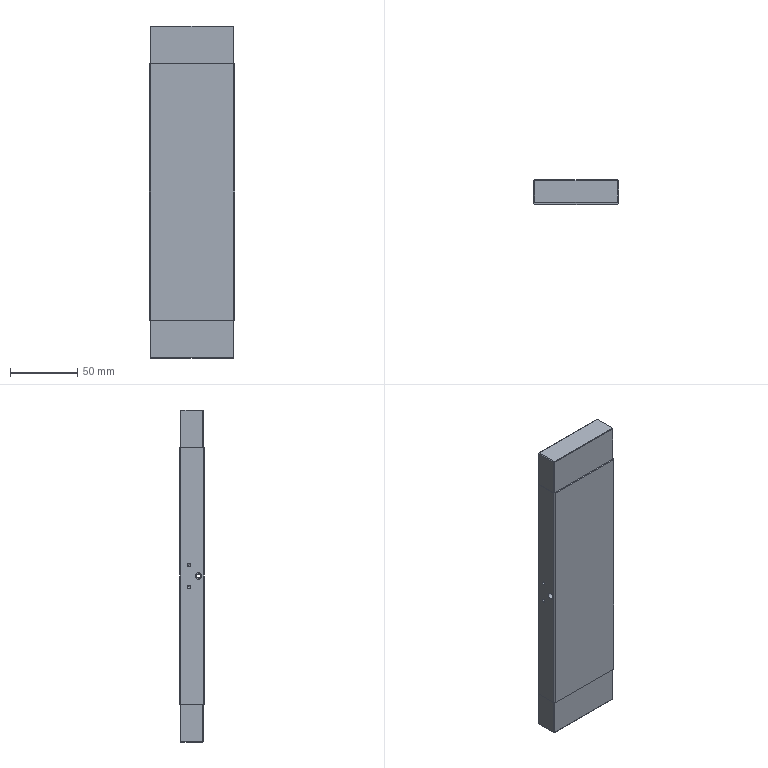Part | SolidWorks | features BaseBody 1 | 1 solid | 148 faces | box 63 x 18.5 x 246 mm | volume 256185 mm3 | plane 77 | cylinder 43 | cone 28 | commonest cylinder face diameters 5 x24 2.5 x8 10 x8 3 x2 1 x1